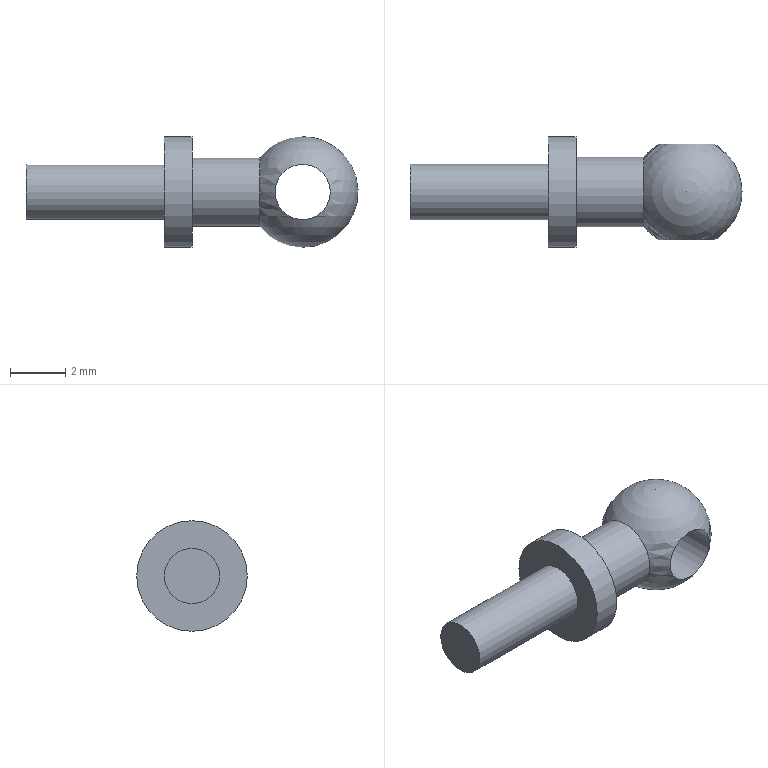Part | STEP file | 1-56.23 | 1 solid | 8 faces | box 12 x 4 x 4 mm | volume 60.89 mm3 | cylinder 4 | plane 3 | sphere 1 | commonest cylinder face diameters 2 x2 2.5 x1 4 x1
STEP:
#1=CARTESIAN_POINT('',(0.,0.,0.));
#2=DIRECTION('',(0.,0.,1.));
#3=DIRECTION('',(1.,0.,0.));
#4=AXIS2_PLACEMENT_3D('',#1,#2,#3);
#5=CARTESIAN_POINT('',(-1.561,1.25,0.));
#6=VERTEX_POINT('',#5);
#7=CARTESIAN_POINT('',(-4.,1.25,0.));
#8=VERTEX_POINT('',#7);
#9=CARTESIAN_POINT('',(-1.561,1.25,0.));
#10=DIRECTION('',(-1.,0.,0.));
#11=VECTOR('',#10,1.);
#12=LINE('',#9,#11);
#13=CARTESIAN_POINT('',(0.,0.,0.));
#14=DIRECTION('',(-1.,0.,0.));
#15=DIRECTION('',(0.,1.,0.));
#16=AXIS2_PLACEMENT_3D('',#13,#14,#15);
#17=CYLINDRICAL_SURFACE('',#16,1.25);
#18=CARTESIAN_POINT('',(0.,1.561));
#19=DIRECTION('',(0.,1.));
#20=VECTOR('',#19,1.);
#21=LINE('',#18,#20);
#22=(GEOMETRIC_REPRESENTATION_CONTEXT(2)PARAMETRIC_REPRESENTATION_CONTEXT()REPRESENTATION_CONTEXT('',''));
#23=DEFINITIONAL_REPRESENTATION('',(#21),#22);
#24=PCURVE('',#17,#23);
#25=CARTESIAN_POINT('',(6.283,1.561));
#26=DIRECTION('',(0.,1.));
#27=VECTOR('',#26,1.);
#28=LINE('',#25,#27);
#29=(GEOMETRIC_REPRESENTATION_CONTEXT(2)PARAMETRIC_REPRESENTATION_CONTEXT()REPRESENTATION_CONTEXT('',''));
#30=DEFINITIONAL_REPRESENTATION('',(#28),#29);
#31=PCURVE('',#17,#30);
#32=SEAM_CURVE('',#12,(#24,#31),.PCURVE_S1.);
#33=EDGE_CURVE('',#6,#8,#32,.T.);
#34=ORIENTED_EDGE('',*,*,#33,.F.);
#35=CARTESIAN_POINT('',(-1.561,0.,0.));
#36=DIRECTION('',(-1.,0.,0.));
#37=DIRECTION('',(0.,1.,0.));
#38=AXIS2_PLACEMENT_3D('',#35,#36,#37);
#39=CIRCLE('',#38,1.25);
#40=CARTESIAN_POINT('',(0.,1.561));
#41=DIRECTION('',(1.,0.));
#42=VECTOR('',#41,1.);
#43=LINE('',#40,#42);
#44=(GEOMETRIC_REPRESENTATION_CONTEXT(2)PARAMETRIC_REPRESENTATION_CONTEXT()REPRESENTATION_CONTEXT('',''));
#45=DEFINITIONAL_REPRESENTATION('',(#43),#44);
#46=PCURVE('',#17,#45);
#47=CARTESIAN_POINT('',(0.,0.,0.));
#48=DIRECTION('',(0.,0.,1.));
#49=DIRECTION('',(1.,0.,0.));
#50=AXIS2_PLACEMENT_3D('',#47,#48,#49);
#51=SPHERICAL_SURFACE('',#50,2.);
#52=CARTESIAN_POINT('',(2.466,0.));
#53=CARTESIAN_POINT('',(2.467,-0.05932));
#54=CARTESIAN_POINT('',(2.479,-0.1786));
#55=CARTESIAN_POINT('',(2.541,-0.348));
#56=CARTESIAN_POINT('',(2.65,-0.4976));
#57=CARTESIAN_POINT('',(2.812,-0.6132));
#58=CARTESIAN_POINT('',(3.024,-0.6778));
#59=CARTESIAN_POINT('',(3.259,-0.6778));
#60=CARTESIAN_POINT('',(3.471,-0.6132));
#61=CARTESIAN_POINT('',(3.633,-0.4976));
#62=CARTESIAN_POINT('',(3.742,-0.348));
#63=CARTESIAN_POINT('',(3.804,-0.1785));
#64=CARTESIAN_POINT('',(3.823,0.));
#65=CARTESIAN_POINT('',(3.804,0.1785));
#66=CARTESIAN_POINT('',(3.742,0.348));
#67=CARTESIAN_POINT('',(3.633,0.4976));
#68=CARTESIAN_POINT('',(3.471,0.6132));
#69=CARTESIAN_POINT('',(3.259,0.6778));
#70=CARTESIAN_POINT('',(3.024,0.6778));
#71=CARTESIAN_POINT('',(2.812,0.6132));
#72=CARTESIAN_POINT('',(2.65,0.4976));
#73=CARTESIAN_POINT('',(2.541,0.348));
#74=CARTESIAN_POINT('',(2.479,0.1786));
#75=CARTESIAN_POINT('',(2.467,0.05932));
#76=CARTESIAN_POINT('',(2.466,0.));
#77=B_SPLINE_CURVE_WITH_KNOTS('',3,(#52,#53,#54,#55,#56,#57,#58,#59,#60,#61,#62,#63,#64,#65,#66,#67,#68,#69,#70,#71,#72,#73,#74,#75,#76),.UNSPECIFIED.,.F.,.F.,(4,1,1,1,1,1,1,1,1,1,1,1,1,1,1,1,1,1,1,1,1,1,4),(0.,0.2856,0.5712,0.8568,1.142,1.428,1.714,1.999,2.285,2.57,2.856,3.142,3.427,3.713,3.998,4.284,4.57,4.855,5.141,5.426,5.712,5.998,6.283),.QUASI_UNIFORM_KNOTS.);
#78=(GEOMETRIC_REPRESENTATION_CONTEXT(2)PARAMETRIC_REPRESENTATION_CONTEXT()REPRESENTATION_CONTEXT('',''));
#79=DEFINITIONAL_REPRESENTATION('',(#77),#78);
#80=PCURVE('',#51,#79);
#81=SURFACE_CURVE('',#39,(#46,#80),.PCURVE_S1.);
#82=EDGE_CURVE('',#6,#6,#81,.T.);
#83=ORIENTED_EDGE('',*,*,#82,.T.);
#84=ORIENTED_EDGE('',*,*,#33,.T.);
#85=CARTESIAN_POINT('',(-4.,0.,0.));
#86=DIRECTION('',(1.,0.,0.));
#87=DIRECTION('',(0.,1.,0.));
#88=AXIS2_PLACEMENT_3D('',#85,#86,#87);
#89=CIRCLE('',#88,1.25);
#90=CARTESIAN_POINT('',(6.283,4.));
#91=DIRECTION('',(-1.,0.));
#92=VECTOR('',#91,1.);
#93=LINE('',#90,#92);
#94=(GEOMETRIC_REPRESENTATION_CONTEXT(2)PARAMETRIC_REPRESENTATION_CONTEXT()REPRESENTATION_CONTEXT('',''));
#95=DEFINITIONAL_REPRESENTATION('',(#93),#94);
#96=PCURVE('',#17,#95);
#97=CARTESIAN_POINT('',(-4.,-0.5359,0.));
#98=DIRECTION('',(1.,0.,0.));
#99=DIRECTION('',(0.,0.,-1.));
#100=AXIS2_PLACEMENT_3D('',#97,#98,#99);
#101=PLANE('',#100);
#102=CARTESIAN_POINT('',(0.,0.5359));
#103=DIRECTION('',(0.,1.));
#104=AXIS2_PLACEMENT_2D('',#102,#103);
#105=CIRCLE('',#104,1.25);
#106=(GEOMETRIC_REPRESENTATION_CONTEXT(2)PARAMETRIC_REPRESENTATION_CONTEXT()REPRESENTATION_CONTEXT('',''));
#107=DEFINITIONAL_REPRESENTATION('',(#105),#106);
#108=PCURVE('',#101,#107);
#109=SURFACE_CURVE('',#89,(#96,#108),.PCURVE_S1.);
#110=EDGE_CURVE('',#8,#8,#109,.T.);
#111=ORIENTED_EDGE('',*,*,#110,.T.);
#112=EDGE_LOOP('',(#34,#83,#84,#111));
#113=FACE_BOUND('',#112,.T.);
#114=ADVANCED_FACE('',(#113),#17,.T.);
#115=CARTESIAN_POINT('',(-4.,2.,0.));
#116=VERTEX_POINT('',#115);
#117=CARTESIAN_POINT('',(-4.,0.,0.));
#118=DIRECTION('',(1.,0.,0.));
#119=DIRECTION('',(0.,1.,0.));
#120=AXIS2_PLACEMENT_3D('',#117,#118,#119);
#121=CIRCLE('',#120,2.);
#122=CARTESIAN_POINT('',(0.,0.5359));
#123=DIRECTION('',(0.,1.));
#124=AXIS2_PLACEMENT_2D('',#122,#123);
#125=CIRCLE('',#124,2.);
#126=(GEOMETRIC_REPRESENTATION_CONTEXT(2)PARAMETRIC_REPRESENTATION_CONTEXT()REPRESENTATION_CONTEXT('',''));
#127=DEFINITIONAL_REPRESENTATION('',(#125),#126);
#128=PCURVE('',#101,#127);
#129=CARTESIAN_POINT('',(-4.,0.,0.));
#130=DIRECTION('',(-1.,0.,0.));
#131=DIRECTION('',(0.,1.,0.));
#132=AXIS2_PLACEMENT_3D('',#129,#130,#131);
#133=CYLINDRICAL_SURFACE('',#132,2.);
#134=CARTESIAN_POINT('',(6.283,0.));
#135=DIRECTION('',(-1.,0.));
#136=VECTOR('',#135,1.);
#137=LINE('',#134,#136);
#138=(GEOMETRIC_REPRESENTATION_CONTEXT(2)PARAMETRIC_REPRESENTATION_CONTEXT()REPRESENTATION_CONTEXT('',''));
#139=DEFINITIONAL_REPRESENTATION('',(#137),#138);
#140=PCURVE('',#133,#139);
#141=SURFACE_CURVE('',#121,(#128,#140),.PCURVE_S1.);
#142=EDGE_CURVE('',#116,#116,#141,.T.);
#143=ORIENTED_EDGE('',*,*,#142,.T.);
#144=EDGE_LOOP('',(#143));
#145=FACE_BOUND('',#144,.T.);
#146=ORIENTED_EDGE('',*,*,#110,.F.);
#147=EDGE_LOOP('',(#146));
#148=FACE_BOUND('',#147,.T.);
#149=ADVANCED_FACE('',(#145,#148),#101,.T.);
#150=CARTESIAN_POINT('',(-5.,2.,0.));
#151=VERTEX_POINT('',#150);
#152=CARTESIAN_POINT('',(-4.,2.,0.));
#153=DIRECTION('',(-1.,0.,0.));
#154=VECTOR('',#153,1.);
#155=LINE('',#152,#154);
#156=CARTESIAN_POINT('',(6.283,0.));
#157=DIRECTION('',(0.,1.));
#158=VECTOR('',#157,1.);
#159=LINE('',#156,#158);
#160=(GEOMETRIC_REPRESENTATION_CONTEXT(2)PARAMETRIC_REPRESENTATION_CONTEXT()REPRESENTATION_CONTEXT('',''));
#161=DEFINITIONAL_REPRESENTATION('',(#159),#160);
#162=PCURVE('',#133,#161);
#163=CARTESIAN_POINT('',(0.,0.));
#164=DIRECTION('',(0.,1.));
#165=VECTOR('',#164,1.);
#166=LINE('',#163,#165);
#167=(GEOMETRIC_REPRESENTATION_CONTEXT(2)PARAMETRIC_REPRESENTATION_CONTEXT()REPRESENTATION_CONTEXT('',''));
#168=DEFINITIONAL_REPRESENTATION('',(#166),#167);
#169=PCURVE('',#133,#168);
#170=SEAM_CURVE('',#155,(#162,#169),.PCURVE_S1.);
#171=EDGE_CURVE('',#116,#151,#170,.T.);
#172=ORIENTED_EDGE('',*,*,#171,.T.);
#173=CARTESIAN_POINT('',(-5.,0.,0.));
#174=DIRECTION('',(1.,0.,0.));
#175=DIRECTION('',(0.,1.,0.));
#176=AXIS2_PLACEMENT_3D('',#173,#174,#175);
#177=CIRCLE('',#176,2.);
#178=CARTESIAN_POINT('',(6.283,1.));
#179=DIRECTION('',(-1.,0.));
#180=VECTOR('',#179,1.);
#181=LINE('',#178,#180);
#182=(GEOMETRIC_REPRESENTATION_CONTEXT(2)PARAMETRIC_REPRESENTATION_CONTEXT()REPRESENTATION_CONTEXT('',''));
#183=DEFINITIONAL_REPRESENTATION('',(#181),#182);
#184=PCURVE('',#133,#183);
#185=CARTESIAN_POINT('',(-5.,-0.5359,0.));
#186=DIRECTION('',(1.,0.,0.));
#187=DIRECTION('',(0.,0.,-1.));
#188=AXIS2_PLACEMENT_3D('',#185,#186,#187);
#189=PLANE('',#188);
#190=CARTESIAN_POINT('',(0.,0.5359));
#191=DIRECTION('',(0.,1.));
#192=AXIS2_PLACEMENT_2D('',#190,#191);
#193=CIRCLE('',#192,2.);
#194=(GEOMETRIC_REPRESENTATION_CONTEXT(2)PARAMETRIC_REPRESENTATION_CONTEXT()REPRESENTATION_CONTEXT('',''));
#195=DEFINITIONAL_REPRESENTATION('',(#193),#194);
#196=PCURVE('',#189,#195);
#197=SURFACE_CURVE('',#177,(#184,#196),.PCURVE_S1.);
#198=EDGE_CURVE('',#151,#151,#197,.T.);
#199=ORIENTED_EDGE('',*,*,#198,.T.);
#200=ORIENTED_EDGE('',*,*,#171,.F.);
#201=ORIENTED_EDGE('',*,*,#142,.F.);
#202=EDGE_LOOP('',(#172,#199,#200,#201));
#203=FACE_BOUND('',#202,.T.);
#204=ADVANCED_FACE('',(#203),#133,.T.);
#205=ORIENTED_EDGE('',*,*,#198,.T.);
#206=EDGE_LOOP('',(#205));
#207=FACE_BOUND('',#206,.F.);
#208=CARTESIAN_POINT('',(-5.,1.,0.));
#209=VERTEX_POINT('',#208);
#210=CARTESIAN_POINT('',(-5.,0.,0.));
#211=DIRECTION('',(1.,0.,0.));
#212=DIRECTION('',(0.,1.,0.));
#213=AXIS2_PLACEMENT_3D('',#210,#211,#212);
#214=CIRCLE('',#213,1.);
#215=CARTESIAN_POINT('',(0.,0.5359));
#216=DIRECTION('',(0.,1.));
#217=AXIS2_PLACEMENT_2D('',#215,#216);
#218=CIRCLE('',#217,1.);
#219=(GEOMETRIC_REPRESENTATION_CONTEXT(2)PARAMETRIC_REPRESENTATION_CONTEXT()REPRESENTATION_CONTEXT('',''));
#220=DEFINITIONAL_REPRESENTATION('',(#218),#219);
#221=PCURVE('',#189,#220);
#222=CARTESIAN_POINT('',(-5.,0.,0.));
#223=DIRECTION('',(-1.,0.,0.));
#224=DIRECTION('',(0.,1.,0.));
#225=AXIS2_PLACEMENT_3D('',#222,#223,#224);
#226=CYLINDRICAL_SURFACE('',#225,1.);
#227=CARTESIAN_POINT('',(6.283,0.));
#228=DIRECTION('',(-1.,0.));
#229=VECTOR('',#228,1.);
#230=LINE('',#227,#229);
#231=(GEOMETRIC_REPRESENTATION_CONTEXT(2)PARAMETRIC_REPRESENTATION_CONTEXT()REPRESENTATION_CONTEXT('',''));
#232=DEFINITIONAL_REPRESENTATION('',(#230),#231);
#233=PCURVE('',#226,#232);
#234=SURFACE_CURVE('',#214,(#221,#233),.PCURVE_S1.);
#235=EDGE_CURVE('',#209,#209,#234,.T.);
#236=ORIENTED_EDGE('',*,*,#235,.F.);
#237=EDGE_LOOP('',(#236));
#238=FACE_BOUND('',#237,.F.);
#239=ADVANCED_FACE('',(#207,#238),#189,.F.);
#240=CARTESIAN_POINT('',(-10.,1.,0.));
#241=VERTEX_POINT('',#240);
#242=CARTESIAN_POINT('',(-5.,1.,0.));
#243=DIRECTION('',(-1.,0.,0.));
#244=VECTOR('',#243,1.);
#245=LINE('',#242,#244);
#246=CARTESIAN_POINT('',(6.283,0.));
#247=DIRECTION('',(0.,1.));
#248=VECTOR('',#247,1.);
#249=LINE('',#246,#248);
#250=(GEOMETRIC_REPRESENTATION_CONTEXT(2)PARAMETRIC_REPRESENTATION_CONTEXT()REPRESENTATION_CONTEXT('',''));
#251=DEFINITIONAL_REPRESENTATION('',(#249),#250);
#252=PCURVE('',#226,#251);
#253=CARTESIAN_POINT('',(0.,0.));
#254=DIRECTION('',(0.,1.));
#255=VECTOR('',#254,1.);
#256=LINE('',#253,#255);
#257=(GEOMETRIC_REPRESENTATION_CONTEXT(2)PARAMETRIC_REPRESENTATION_CONTEXT()REPRESENTATION_CONTEXT('',''));
#258=DEFINITIONAL_REPRESENTATION('',(#256),#257);
#259=PCURVE('',#226,#258);
#260=SEAM_CURVE('',#245,(#252,#259),.PCURVE_S1.);
#261=EDGE_CURVE('',#209,#241,#260,.T.);
#262=ORIENTED_EDGE('',*,*,#261,.T.);
#263=CARTESIAN_POINT('',(-10.,0.,0.));
#264=DIRECTION('',(1.,0.,0.));
#265=DIRECTION('',(0.,1.,0.));
#266=AXIS2_PLACEMENT_3D('',#263,#264,#265);
#267=CIRCLE('',#266,1.);
#268=CARTESIAN_POINT('',(6.283,5.));
#269=DIRECTION('',(-1.,0.));
#270=VECTOR('',#269,1.);
#271=LINE('',#268,#270);
#272=(GEOMETRIC_REPRESENTATION_CONTEXT(2)PARAMETRIC_REPRESENTATION_CONTEXT()REPRESENTATION_CONTEXT('',''));
#273=DEFINITIONAL_REPRESENTATION('',(#271),#272);
#274=PCURVE('',#226,#273);
#275=CARTESIAN_POINT('',(-10.,-0.2679,0.));
#276=DIRECTION('',(1.,0.,0.));
#277=DIRECTION('',(0.,0.,-1.));
#278=AXIS2_PLACEMENT_3D('',#275,#276,#277);
#279=PLANE('',#278);
#280=CARTESIAN_POINT('',(0.,0.2679));
#281=DIRECTION('',(0.,1.));
#282=AXIS2_PLACEMENT_2D('',#280,#281);
#283=CIRCLE('',#282,1.);
#284=(GEOMETRIC_REPRESENTATION_CONTEXT(2)PARAMETRIC_REPRESENTATION_CONTEXT()REPRESENTATION_CONTEXT('',''));
#285=DEFINITIONAL_REPRESENTATION('',(#283),#284);
#286=PCURVE('',#279,#285);
#287=SURFACE_CURVE('',#267,(#274,#286),.PCURVE_S1.);
#288=EDGE_CURVE('',#241,#241,#287,.T.);
#289=ORIENTED_EDGE('',*,*,#288,.T.);
#290=ORIENTED_EDGE('',*,*,#261,.F.);
#291=ORIENTED_EDGE('',*,*,#235,.F.);
#292=EDGE_LOOP('',(#262,#289,#290,#291));
#293=FACE_BOUND('',#292,.T.);
#294=ADVANCED_FACE('',(#293),#226,.T.);
#295=ORIENTED_EDGE('',*,*,#288,.T.);
#296=EDGE_LOOP('',(#295));
#297=FACE_BOUND('',#296,.F.);
#298=ADVANCED_FACE('',(#297),#279,.F.);
#299=CARTESIAN_POINT('',(0.,0.,2.));
#300=VERTEX_POINT('',#299);
#301=VERTEX_LOOP('',#300);
#302=FACE_BOUND('',#301,.T.);
#303=CARTESIAN_POINT('',(1.,1.732,0.));
#304=VERTEX_POINT('',#303);
#305=CARTESIAN_POINT('',(0.,1.732,0.));
#306=DIRECTION('',(0.,1.,0.));
#307=DIRECTION('',(1.,0.,0.));
#308=AXIS2_PLACEMENT_3D('',#305,#306,#307);
#309=CIRCLE('',#308,1.);
#310=CARTESIAN_POINT('',(1.047,0.));
#311=CARTESIAN_POINT('',(1.047,-0.04753));
#312=CARTESIAN_POINT('',(1.059,-0.1428));
#313=CARTESIAN_POINT('',(1.112,-0.2768));
#314=CARTESIAN_POINT('',(1.203,-0.3924));
#315=CARTESIAN_POINT('',(1.331,-0.4788));
#316=CARTESIAN_POINT('',(1.487,-0.5255));
#317=CARTESIAN_POINT('',(1.655,-0.5255));
#318=CARTESIAN_POINT('',(1.811,-0.4788));
#319=CARTESIAN_POINT('',(1.938,-0.3924));
#320=CARTESIAN_POINT('',(2.029,-0.2768));
#321=CARTESIAN_POINT('',(2.083,-0.1428));
#322=CARTESIAN_POINT('',(2.1,0.));
#323=CARTESIAN_POINT('',(2.083,0.1428));
#324=CARTESIAN_POINT('',(2.029,0.2768));
#325=CARTESIAN_POINT('',(1.938,0.3924));
#326=CARTESIAN_POINT('',(1.811,0.4788));
#327=CARTESIAN_POINT('',(1.655,0.5255));
#328=CARTESIAN_POINT('',(1.487,0.5255));
#329=CARTESIAN_POINT('',(1.331,0.4788));
#330=CARTESIAN_POINT('',(1.203,0.3924));
#331=CARTESIAN_POINT('',(1.112,0.2768));
#332=CARTESIAN_POINT('',(1.059,0.1428));
#333=CARTESIAN_POINT('',(1.047,0.04753));
#334=CARTESIAN_POINT('',(1.047,0.));
#335=B_SPLINE_CURVE_WITH_KNOTS('',3,(#310,#311,#312,#313,#314,#315,#316,#317,#318,#319,#320,#321,#322,#323,#324,#325,#326,#327,#328,#329,#330,#331,#332,#333,#334),.UNSPECIFIED.,.F.,.F.,(4,1,1,1,1,1,1,1,1,1,1,1,1,1,1,1,1,1,1,1,1,1,4),(0.,0.2856,0.5712,0.8568,1.142,1.428,1.714,1.999,2.285,2.57,2.856,3.142,3.427,3.713,3.998,4.284,4.57,4.855,5.141,5.426,5.712,5.998,6.283),.QUASI_UNIFORM_KNOTS.);
#336=(GEOMETRIC_REPRESENTATION_CONTEXT(2)PARAMETRIC_REPRESENTATION_CONTEXT()REPRESENTATION_CONTEXT('',''));
#337=DEFINITIONAL_REPRESENTATION('',(#335),#336);
#338=PCURVE('',#51,#337);
#339=CARTESIAN_POINT('',(0.,-6.5,0.));
#340=DIRECTION('',(0.,1.,0.));
#341=DIRECTION('',(1.,0.,0.));
#342=AXIS2_PLACEMENT_3D('',#339,#340,#341);
#343=CYLINDRICAL_SURFACE('',#342,1.);
#344=CARTESIAN_POINT('',(0.,8.232));
#345=DIRECTION('',(1.,0.));
#346=VECTOR('',#345,1.);
#347=LINE('',#344,#346);
#348=(GEOMETRIC_REPRESENTATION_CONTEXT(2)PARAMETRIC_REPRESENTATION_CONTEXT()REPRESENTATION_CONTEXT('',''));
#349=DEFINITIONAL_REPRESENTATION('',(#347),#348);
#350=PCURVE('',#343,#349);
#351=SURFACE_CURVE('',#309,(#338,#350),.PCURVE_S1.);
#352=EDGE_CURVE('',#304,#304,#351,.T.);
#353=ORIENTED_EDGE('',*,*,#352,.F.);
#354=EDGE_LOOP('',(#353));
#355=FACE_BOUND('',#354,.T.);
#356=CARTESIAN_POINT('',(1.,-1.732,0.));
#357=VERTEX_POINT('',#356);
#358=CARTESIAN_POINT('',(0.,-1.732,0.));
#359=DIRECTION('',(0.,-1.,0.));
#360=DIRECTION('',(1.,0.,0.));
#361=AXIS2_PLACEMENT_3D('',#358,#359,#360);
#362=CIRCLE('',#361,1.);
#363=CARTESIAN_POINT('',(5.236,0.));
#364=CARTESIAN_POINT('',(5.236,0.04753));
#365=CARTESIAN_POINT('',(5.224,0.1428));
#366=CARTESIAN_POINT('',(5.171,0.2768));
#367=CARTESIAN_POINT('',(5.08,0.3924));
#368=CARTESIAN_POINT('',(4.953,0.4788));
#369=CARTESIAN_POINT('',(4.796,0.5255));
#370=CARTESIAN_POINT('',(4.629,0.5255));
#371=CARTESIAN_POINT('',(4.472,0.4788));
#372=CARTESIAN_POINT('',(4.345,0.3924));
#373=CARTESIAN_POINT('',(4.254,0.2768));
#374=CARTESIAN_POINT('',(4.201,0.1428));
#375=CARTESIAN_POINT('',(4.183,0.));
#376=CARTESIAN_POINT('',(4.201,-0.1428));
#377=CARTESIAN_POINT('',(4.254,-0.2768));
#378=CARTESIAN_POINT('',(4.345,-0.3924));
#379=CARTESIAN_POINT('',(4.472,-0.4788));
#380=CARTESIAN_POINT('',(4.629,-0.5255));
#381=CARTESIAN_POINT('',(4.796,-0.5255));
#382=CARTESIAN_POINT('',(4.953,-0.4788));
#383=CARTESIAN_POINT('',(5.08,-0.3924));
#384=CARTESIAN_POINT('',(5.171,-0.2768));
#385=CARTESIAN_POINT('',(5.224,-0.1428));
#386=CARTESIAN_POINT('',(5.236,-0.04753));
#387=CARTESIAN_POINT('',(5.236,0.));
#388=B_SPLINE_CURVE_WITH_KNOTS('',3,(#363,#364,#365,#366,#367,#368,#369,#370,#371,#372,#373,#374,#375,#376,#377,#378,#379,#380,#381,#382,#383,#384,#385,#386,#387),.UNSPECIFIED.,.F.,.F.,(4,1,1,1,1,1,1,1,1,1,1,1,1,1,1,1,1,1,1,1,1,1,4),(0.,0.2856,0.5712,0.8568,1.142,1.428,1.714,1.999,2.285,2.57,2.856,3.142,3.427,3.713,3.998,4.284,4.57,4.855,5.141,5.426,5.712,5.998,6.283),.QUASI_UNIFORM_KNOTS.);
#389=(GEOMETRIC_REPRESENTATION_CONTEXT(2)PARAMETRIC_REPRESENTATION_CONTEXT()REPRESENTATION_CONTEXT('',''));
#390=DEFINITIONAL_REPRESENTATION('',(#388),#389);
#391=PCURVE('',#51,#390);
#392=CARTESIAN_POINT('',(6.283,4.768));
#393=DIRECTION('',(-1.,0.));
#394=VECTOR('',#393,1.);
#395=LINE('',#392,#394);
#396=(GEOMETRIC_REPRESENTATION_CONTEXT(2)PARAMETRIC_REPRESENTATION_CONTEXT()REPRESENTATION_CONTEXT('',''));
#397=DEFINITIONAL_REPRESENTATION('',(#395),#396);
#398=PCURVE('',#343,#397);
#399=SURFACE_CURVE('',#362,(#391,#398),.PCURVE_S1.);
#400=EDGE_CURVE('',#357,#357,#399,.T.);
#401=ORIENTED_EDGE('',*,*,#400,.F.);
#402=EDGE_LOOP('',(#401));
#403=FACE_BOUND('',#402,.T.);
#404=ORIENTED_EDGE('',*,*,#82,.F.);
#405=EDGE_LOOP('',(#404));
#406=FACE_BOUND('',#405,.T.);
#407=ADVANCED_FACE('',(#302,#355,#403,#406),#51,.T.);
#408=ORIENTED_EDGE('',*,*,#400,.F.);
#409=CARTESIAN_POINT('',(1.,-1.732,0.));
#410=DIRECTION('',(0.,1.,0.));
#411=VECTOR('',#410,1.);
#412=LINE('',#409,#411);
#413=CARTESIAN_POINT('',(6.283,4.768));
#414=DIRECTION('',(0.,1.));
#415=VECTOR('',#414,1.);
#416=LINE('',#413,#415);
#417=(GEOMETRIC_REPRESENTATION_CONTEXT(2)PARAMETRIC_REPRESENTATION_CONTEXT()REPRESENTATION_CONTEXT('',''));
#418=DEFINITIONAL_REPRESENTATION('',(#416),#417);
#419=PCURVE('',#343,#418);
#420=CARTESIAN_POINT('',(0.,4.768));
#421=DIRECTION('',(0.,1.));
#422=VECTOR('',#421,1.);
#423=LINE('',#420,#422);
#424=(GEOMETRIC_REPRESENTATION_CONTEXT(2)PARAMETRIC_REPRESENTATION_CONTEXT()REPRESENTATION_CONTEXT('',''));
#425=DEFINITIONAL_REPRESENTATION('',(#423),#424);
#426=PCURVE('',#343,#425);
#427=SEAM_CURVE('',#412,(#419,#426),.PCURVE_S1.);
#428=EDGE_CURVE('',#357,#304,#427,.T.);
#429=ORIENTED_EDGE('',*,*,#428,.T.);
#430=ORIENTED_EDGE('',*,*,#352,.F.);
#431=ORIENTED_EDGE('',*,*,#428,.F.);
#432=EDGE_LOOP('',(#408,#429,#430,#431));
#433=FACE_BOUND('',#432,.F.);
#434=ADVANCED_FACE('',(#433),#343,.F.);
#435=CLOSED_SHELL('',(#114,#149,#204,#239,#294,#298,#407,#434));
#436=MANIFOLD_SOLID_BREP('',#435);
#437=(LENGTH_UNIT()NAMED_UNIT(*)SI_UNIT(.MILLI.,.METRE.));
#438=UNCERTAINTY_MEASURE_WITH_UNIT(LENGTH_MEASURE(0.0000001),#437,'','');
#439=(NAMED_UNIT(*)PLANE_ANGLE_UNIT()SI_UNIT($,.RADIAN.));
#440=(NAMED_UNIT(*)SI_UNIT($,.STERADIAN.)SOLID_ANGLE_UNIT());
#441=(GEOMETRIC_REPRESENTATION_CONTEXT(3)GLOBAL_UNCERTAINTY_ASSIGNED_CONTEXT((#438))GLOBAL_UNIT_ASSIGNED_CONTEXT((#437,#439,#440))REPRESENTATION_CONTEXT('',''));
#442=ADVANCED_BREP_SHAPE_REPRESENTATION('',(#4,#436),#441);